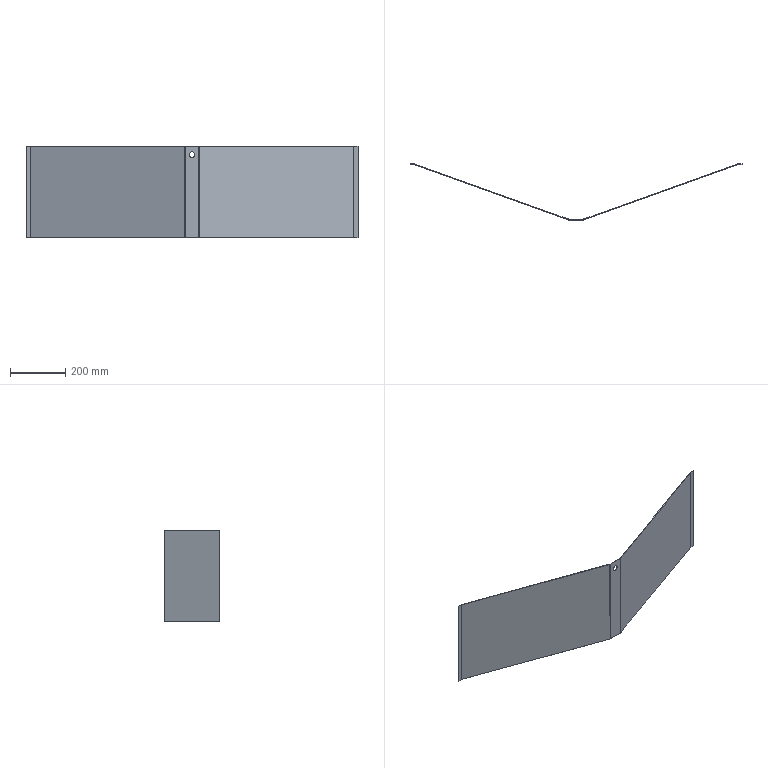Part | SolidWorks | features ICE 2, Fillet 1, FlatPattern 1, SMBaseFlange 1, SheetMetal 1 | 1 solid | 40 faces | box 1200 x 202 x 330 mm | volume 837082 mm3 | plane 30 | cylinder 10 | commonest cylinder face diameters 2 x4 6 x4 20 x2
STEP:
#1=CARTESIAN_POINT('',(600.,-200.,290.));
#2=VERTEX_POINT('',#1);
#3=CARTESIAN_POINT('',(600.,-200.,310.));
#4=VERTEX_POINT('',#3);
#5=CARTESIAN_POINT('',(600.,-200.,300.));
#6=DIRECTION('',(0.,1.,0.));
#7=DIRECTION('',(0.,0.,1.));
#8=AXIS2_PLACEMENT_3D('',#5,#6,#7);
#9=CIRCLE('',#8,10.);
#10=EDGE_CURVE('',#2,#4,#9,.T.);
#11=ORIENTED_EDGE('',*,*,#10,.T.);
#12=CARTESIAN_POINT('',(600.,-202.,310.));
#13=VERTEX_POINT('',#12);
#14=CARTESIAN_POINT('',(600.,-192.,310.));
#15=DIRECTION('',(0.,-1.,0.));
#16=VECTOR('',#15,1000.);
#17=LINE('',#14,#16);
#18=EDGE_CURVE('',#4,#13,#17,.T.);
#19=ORIENTED_EDGE('',*,*,#18,.T.);
#20=CARTESIAN_POINT('',(600.,-202.,290.));
#21=VERTEX_POINT('',#20);
#22=CARTESIAN_POINT('',(600.,-202.,300.));
#23=DIRECTION('',(0.,-1.,0.));
#24=DIRECTION('',(0.,0.,-1.));
#25=AXIS2_PLACEMENT_3D('',#22,#23,#24);
#26=CIRCLE('',#25,10.);
#27=EDGE_CURVE('',#13,#21,#26,.T.);
#28=ORIENTED_EDGE('',*,*,#27,.T.);
#29=CARTESIAN_POINT('',(600.,-192.,290.));
#30=DIRECTION('',(0.,-1.,0.));
#31=VECTOR('',#30,1000.);
#32=LINE('',#29,#31);
#33=EDGE_CURVE('',#2,#21,#32,.T.);
#34=ORIENTED_EDGE('',*,*,#33,.F.);
#35=EDGE_LOOP('',(#11,#19,#28,#34));
#36=FACE_OUTER_BOUND('',#35,.T.);
#37=CARTESIAN_POINT('',(600.,-192.,300.));
#38=DIRECTION('',(0.,-1.,0.));
#39=DIRECTION('',(0.,0.,-1.));
#40=AXIS2_PLACEMENT_3D('',#37,#38,#39);
#41=CYLINDRICAL_SURFACE('',#40,10.);
#42=ADVANCED_FACE('',(#36),#41,.F.);
#43=CARTESIAN_POINT('',(15.489,-0.1748,330.));
#44=VERTEX_POINT('',#43);
#45=CARTESIAN_POINT('',(14.817,-2.058,330.));
#46=VERTEX_POINT('',#45);
#47=CARTESIAN_POINT('',(15.489,-0.1748,330.));
#48=DIRECTION('',(-0.3363,-0.9417,0.));
#49=VECTOR('',#48,1000.);
#50=LINE('',#47,#49);
#51=EDGE_CURVE('',#44,#46,#50,.T.);
#52=ORIENTED_EDGE('',*,*,#51,.F.);
#53=CARTESIAN_POINT('',(14.48,0.,330.));
#54=VERTEX_POINT('',#53);
#55=CARTESIAN_POINT('',(14.48,-3.,330.));
#56=DIRECTION('',(0.,0.,-1.));
#57=DIRECTION('',(1.,0.,0.));
#58=AXIS2_PLACEMENT_3D('',#55,#56,#57);
#59=CIRCLE('',#58,3.);
#60=EDGE_CURVE('',#54,#44,#59,.T.);
#61=ORIENTED_EDGE('',*,*,#60,.F.);
#62=CARTESIAN_POINT('',(14.48,-2.,330.));
#63=VERTEX_POINT('',#62);
#64=CARTESIAN_POINT('',(14.48,-2.,330.));
#65=DIRECTION('',(0.,1.,0.));
#66=VECTOR('',#65,1000.);
#67=LINE('',#64,#66);
#68=EDGE_CURVE('',#63,#54,#67,.T.);
#69=ORIENTED_EDGE('',*,*,#68,.F.);
#70=CARTESIAN_POINT('',(14.48,-3.,330.));
#71=DIRECTION('',(0.,0.,-1.));
#72=DIRECTION('',(1.,0.,0.));
#73=AXIS2_PLACEMENT_3D('',#70,#71,#72);
#74=CIRCLE('',#73,1.);
#75=EDGE_CURVE('',#63,#46,#74,.T.);
#76=ORIENTED_EDGE('',*,*,#75,.T.);
#77=EDGE_LOOP('',(#52,#61,#69,#76));
#78=FACE_OUTER_BOUND('',#77,.T.);
#79=CARTESIAN_POINT('',(15.489,-0.1748,330.));
#80=DIRECTION('',(0.,0.,1.));
#81=DIRECTION('',(1.,0.,0.));
#82=AXIS2_PLACEMENT_3D('',#79,#80,#81);
#83=PLANE('',#82);
#84=ADVANCED_FACE('',(#78),#83,.T.);
#85=CARTESIAN_POINT('',(574.837,-199.942,330.));
#86=VERTEX_POINT('',#85);
#87=CARTESIAN_POINT('',(15.,0.,330.));
#88=DIRECTION('',(0.9417,-0.3363,0.));
#89=VECTOR('',#88,1000.);
#90=LINE('',#87,#89);
#91=EDGE_CURVE('',#44,#86,#90,.T.);
#92=ORIENTED_EDGE('',*,*,#91,.F.);
#93=ORIENTED_EDGE('',*,*,#51,.T.);
#94=CARTESIAN_POINT('',(574.164,-201.825,330.));
#95=VERTEX_POINT('',#94);
#96=CARTESIAN_POINT('',(14.327,-1.883,330.));
#97=DIRECTION('',(0.9417,-0.3363,0.));
#98=VECTOR('',#97,1000.);
#99=LINE('',#96,#98);
#100=EDGE_CURVE('',#46,#95,#99,.T.);
#101=ORIENTED_EDGE('',*,*,#100,.T.);
#102=CARTESIAN_POINT('',(574.164,-201.825,330.));
#103=DIRECTION('',(0.3363,0.9417,0.));
#104=VECTOR('',#103,1000.);
#105=LINE('',#102,#104);
#106=EDGE_CURVE('',#95,#86,#105,.T.);
#107=ORIENTED_EDGE('',*,*,#106,.T.);
#108=EDGE_LOOP('',(#92,#93,#101,#107));
#109=FACE_OUTER_BOUND('',#108,.T.);
#110=CARTESIAN_POINT('',(14.48,-2.,330.));
#111=DIRECTION('',(0.,0.,1.));
#112=DIRECTION('',(1.,0.,0.));
#113=AXIS2_PLACEMENT_3D('',#110,#111,#112);
#114=PLANE('',#113);
#115=ADVANCED_FACE('',(#109),#114,.T.);
#116=CARTESIAN_POINT('',(14.48,0.,0.));
#117=VERTEX_POINT('',#116);
#118=CARTESIAN_POINT('',(14.48,-2.,0.));
#119=VERTEX_POINT('',#118);
#120=CARTESIAN_POINT('',(14.48,0.,0.));
#121=DIRECTION('',(0.,-1.,0.));
#122=VECTOR('',#121,1000.);
#123=LINE('',#120,#122);
#124=EDGE_CURVE('',#117,#119,#123,.T.);
#125=ORIENTED_EDGE('',*,*,#124,.F.);
#126=CARTESIAN_POINT('',(15.489,-0.1748,0.));
#127=VERTEX_POINT('',#126);
#128=CARTESIAN_POINT('',(14.48,-3.,0.));
#129=DIRECTION('',(0.,0.,-1.));
#130=DIRECTION('',(1.,0.,0.));
#131=AXIS2_PLACEMENT_3D('',#128,#129,#130);
#132=CIRCLE('',#131,3.);
#133=EDGE_CURVE('',#117,#127,#132,.T.);
#134=ORIENTED_EDGE('',*,*,#133,.T.);
#135=CARTESIAN_POINT('',(14.817,-2.058,0.));
#136=VERTEX_POINT('',#135);
#137=CARTESIAN_POINT('',(14.817,-2.058,0.));
#138=DIRECTION('',(0.3363,0.9417,0.));
#139=VECTOR('',#138,1000.);
#140=LINE('',#137,#139);
#141=EDGE_CURVE('',#136,#127,#140,.T.);
#142=ORIENTED_EDGE('',*,*,#141,.F.);
#143=CARTESIAN_POINT('',(14.48,-3.,0.));
#144=DIRECTION('',(0.,0.,-1.));
#145=DIRECTION('',(1.,0.,0.));
#146=AXIS2_PLACEMENT_3D('',#143,#144,#145);
#147=CIRCLE('',#146,1.);
#148=EDGE_CURVE('',#119,#136,#147,.T.);
#149=ORIENTED_EDGE('',*,*,#148,.F.);
#150=EDGE_LOOP('',(#125,#134,#142,#149));
#151=FACE_OUTER_BOUND('',#150,.T.);
#152=CARTESIAN_POINT('',(14.48,0.,0.));
#153=DIRECTION('',(0.,0.,-1.));
#154=DIRECTION('',(-1.,0.,0.));
#155=AXIS2_PLACEMENT_3D('',#152,#153,#154);
#156=PLANE('',#155);
#157=ADVANCED_FACE('',(#151),#156,.T.);
#158=CARTESIAN_POINT('',(0.,0.,0.));
#159=VERTEX_POINT('',#158);
#160=CARTESIAN_POINT('',(0.,0.,0.));
#161=DIRECTION('',(1.,0.,0.));
#162=VECTOR('',#161,1000.);
#163=LINE('',#160,#162);
#164=EDGE_CURVE('',#159,#117,#163,.T.);
#165=ORIENTED_EDGE('',*,*,#164,.T.);
#166=ORIENTED_EDGE('',*,*,#124,.T.);
#167=CARTESIAN_POINT('',(0.,-2.,0.));
#168=VERTEX_POINT('',#167);
#169=CARTESIAN_POINT('',(0.,-2.,0.));
#170=DIRECTION('',(1.,0.,0.));
#171=VECTOR('',#170,1000.);
#172=LINE('',#169,#171);
#173=EDGE_CURVE('',#168,#119,#172,.T.);
#174=ORIENTED_EDGE('',*,*,#173,.F.);
#175=CARTESIAN_POINT('',(0.,-2.,0.));
#176=DIRECTION('',(0.,1.,0.));
#177=VECTOR('',#176,1000.);
#178=LINE('',#175,#177);
#179=EDGE_CURVE('',#168,#159,#178,.T.);
#180=ORIENTED_EDGE('',*,*,#179,.T.);
#181=EDGE_LOOP('',(#165,#166,#174,#180));
#182=FACE_OUTER_BOUND('',#181,.T.);
#183=CARTESIAN_POINT('',(14.817,-2.058,0.));
#184=DIRECTION('',(0.,0.,-1.));
#185=DIRECTION('',(-1.,0.,0.));
#186=AXIS2_PLACEMENT_3D('',#183,#184,#185);
#187=PLANE('',#186);
#188=ADVANCED_FACE('',(#182),#187,.T.);
#189=CARTESIAN_POINT('',(575.173,-200.,330.));
#190=VERTEX_POINT('',#189);
#191=CARTESIAN_POINT('',(575.173,-202.,330.));
#192=VERTEX_POINT('',#191);
#193=CARTESIAN_POINT('',(575.173,-200.,330.));
#194=DIRECTION('',(0.,-1.,0.));
#195=VECTOR('',#194,1000.);
#196=LINE('',#193,#195);
#197=EDGE_CURVE('',#190,#192,#196,.T.);
#198=ORIENTED_EDGE('',*,*,#197,.F.);
#199=CARTESIAN_POINT('',(575.173,-199.,330.));
#200=DIRECTION('',(0.,0.,1.));
#201=DIRECTION('',(-1.,0.,0.));
#202=AXIS2_PLACEMENT_3D('',#199,#200,#201);
#203=CIRCLE('',#202,1.);
#204=EDGE_CURVE('',#86,#190,#203,.T.);
#205=ORIENTED_EDGE('',*,*,#204,.F.);
#206=ORIENTED_EDGE('',*,*,#106,.F.);
#207=CARTESIAN_POINT('',(575.173,-199.,330.));
#208=DIRECTION('',(0.,0.,1.));
#209=DIRECTION('',(1.,0.,0.));
#210=AXIS2_PLACEMENT_3D('',#207,#208,#209);
#211=CIRCLE('',#210,3.);
#212=EDGE_CURVE('',#95,#192,#211,.T.);
#213=ORIENTED_EDGE('',*,*,#212,.T.);
#214=EDGE_LOOP('',(#198,#205,#206,#213));
#215=FACE_OUTER_BOUND('',#214,.T.);
#216=CARTESIAN_POINT('',(575.173,-200.,330.));
#217=DIRECTION('',(0.,0.,1.));
#218=DIRECTION('',(1.,0.,0.));
#219=AXIS2_PLACEMENT_3D('',#216,#217,#218);
#220=PLANE('',#219);
#221=ADVANCED_FACE('',(#215),#220,.T.);
#222=CARTESIAN_POINT('',(624.827,-200.,330.));
#223=VERTEX_POINT('',#222);
#224=CARTESIAN_POINT('',(575.,-200.,330.));
#225=DIRECTION('',(1.,0.,0.));
#226=VECTOR('',#225,1000.);
#227=LINE('',#224,#226);
#228=EDGE_CURVE('',#190,#223,#227,.T.);
#229=ORIENTED_EDGE('',*,*,#228,.F.);
#230=ORIENTED_EDGE('',*,*,#197,.T.);
#231=CARTESIAN_POINT('',(624.827,-202.,330.));
#232=VERTEX_POINT('',#231);
#233=CARTESIAN_POINT('',(575.,-202.,330.));
#234=DIRECTION('',(1.,0.,0.));
#235=VECTOR('',#234,1000.);
#236=LINE('',#233,#235);
#237=EDGE_CURVE('',#192,#232,#236,.T.);
#238=ORIENTED_EDGE('',*,*,#237,.T.);
#239=CARTESIAN_POINT('',(624.827,-202.,330.));
#240=DIRECTION('',(0.,1.,0.));
#241=VECTOR('',#240,1000.);
#242=LINE('',#239,#241);
#243=EDGE_CURVE('',#232,#223,#242,.T.);
#244=ORIENTED_EDGE('',*,*,#243,.T.);
#245=EDGE_LOOP('',(#229,#230,#238,#244));
#246=FACE_OUTER_BOUND('',#245,.T.);
#247=CARTESIAN_POINT('',(574.164,-201.825,330.));
#248=DIRECTION('',(0.,0.,1.));
#249=DIRECTION('',(1.,0.,0.));
#250=AXIS2_PLACEMENT_3D('',#247,#248,#249);
#251=PLANE('',#250);
#252=ADVANCED_FACE('',(#246),#251,.T.);
#253=CARTESIAN_POINT('',(574.837,-199.942,0.));
#254=VERTEX_POINT('',#253);
#255=CARTESIAN_POINT('',(574.164,-201.825,0.));
#256=VERTEX_POINT('',#255);
#257=CARTESIAN_POINT('',(574.837,-199.942,0.));
#258=DIRECTION('',(-0.3363,-0.9417,0.));
#259=VECTOR('',#258,1000.);
#260=LINE('',#257,#259);
#261=EDGE_CURVE('',#254,#256,#260,.T.);
#262=ORIENTED_EDGE('',*,*,#261,.F.);
#263=CARTESIAN_POINT('',(575.173,-200.,0.));
#264=VERTEX_POINT('',#263);
#265=CARTESIAN_POINT('',(575.173,-199.,0.));
#266=DIRECTION('',(0.,0.,1.));
#267=DIRECTION('',(-1.,0.,0.));
#268=AXIS2_PLACEMENT_3D('',#265,#266,#267);
#269=CIRCLE('',#268,1.);
#270=EDGE_CURVE('',#254,#264,#269,.T.);
#271=ORIENTED_EDGE('',*,*,#270,.T.);
#272=CARTESIAN_POINT('',(575.173,-202.,0.));
#273=VERTEX_POINT('',#272);
#274=CARTESIAN_POINT('',(575.173,-202.,0.));
#275=DIRECTION('',(0.,1.,0.));
#276=VECTOR('',#275,1000.);
#277=LINE('',#274,#276);
#278=EDGE_CURVE('',#273,#264,#277,.T.);
#279=ORIENTED_EDGE('',*,*,#278,.F.);
#280=CARTESIAN_POINT('',(575.173,-199.,0.));
#281=DIRECTION('',(0.,0.,1.));
#282=DIRECTION('',(1.,0.,0.));
#283=AXIS2_PLACEMENT_3D('',#280,#281,#282);
#284=CIRCLE('',#283,3.);
#285=EDGE_CURVE('',#256,#273,#284,.T.);
#286=ORIENTED_EDGE('',*,*,#285,.F.);
#287=EDGE_LOOP('',(#262,#271,#279,#286));
#288=FACE_OUTER_BOUND('',#287,.T.);
#289=CARTESIAN_POINT('',(574.837,-199.942,0.));
#290=DIRECTION('',(0.,0.,-1.));
#291=DIRECTION('',(-1.,0.,0.));
#292=AXIS2_PLACEMENT_3D('',#289,#290,#291);
#293=PLANE('',#292);
#294=ADVANCED_FACE('',(#288),#293,.T.);
#295=CARTESIAN_POINT('',(15.,0.,0.));
#296=DIRECTION('',(0.9417,-0.3363,0.));
#297=VECTOR('',#296,1000.);
#298=LINE('',#295,#297);
#299=EDGE_CURVE('',#127,#254,#298,.T.);
#300=ORIENTED_EDGE('',*,*,#299,.T.);
#301=ORIENTED_EDGE('',*,*,#261,.T.);
#302=CARTESIAN_POINT('',(14.327,-1.883,0.));
#303=DIRECTION('',(0.9417,-0.3363,0.));
#304=VECTOR('',#303,1000.);
#305=LINE('',#302,#304);
#306=EDGE_CURVE('',#136,#256,#305,.T.);
#307=ORIENTED_EDGE('',*,*,#306,.F.);
#308=ORIENTED_EDGE('',*,*,#141,.T.);
#309=EDGE_LOOP('',(#300,#301,#307,#308));
#310=FACE_OUTER_BOUND('',#309,.T.);
#311=CARTESIAN_POINT('',(575.173,-202.,0.));
#312=DIRECTION('',(0.,0.,-1.));
#313=DIRECTION('',(-1.,0.,0.));
#314=AXIS2_PLACEMENT_3D('',#311,#312,#313);
#315=PLANE('',#314);
#316=ADVANCED_FACE('',(#310),#315,.T.);
#317=CARTESIAN_POINT('',(625.163,-199.942,330.));
#318=VERTEX_POINT('',#317);
#319=CARTESIAN_POINT('',(625.836,-201.825,330.));
#320=VERTEX_POINT('',#319);
#321=CARTESIAN_POINT('',(625.163,-199.942,330.));
#322=DIRECTION('',(0.3363,-0.9417,0.));
#323=VECTOR('',#322,1000.);
#324=LINE('',#321,#323);
#325=EDGE_CURVE('',#318,#320,#324,.T.);
#326=ORIENTED_EDGE('',*,*,#325,.F.);
#327=CARTESIAN_POINT('',(624.827,-199.,330.));
#328=DIRECTION('',(0.,0.,1.));
#329=DIRECTION('',(-1.,0.,0.));
#330=AXIS2_PLACEMENT_3D('',#327,#328,#329);
#331=CIRCLE('',#330,1.);
#332=EDGE_CURVE('',#223,#318,#331,.T.);
#333=ORIENTED_EDGE('',*,*,#332,.F.);
#334=ORIENTED_EDGE('',*,*,#243,.F.);
#335=CARTESIAN_POINT('',(624.827,-199.,330.));
#336=DIRECTION('',(0.,0.,1.));
#337=DIRECTION('',(1.,0.,0.));
#338=AXIS2_PLACEMENT_3D('',#335,#336,#337);
#339=CIRCLE('',#338,3.);
#340=EDGE_CURVE('',#232,#320,#339,.T.);
#341=ORIENTED_EDGE('',*,*,#340,.T.);
#342=EDGE_LOOP('',(#326,#333,#334,#341));
#343=FACE_OUTER_BOUND('',#342,.T.);
#344=CARTESIAN_POINT('',(625.163,-199.942,330.));
#345=DIRECTION('',(0.,0.,1.));
#346=DIRECTION('',(1.,0.,0.));
#347=AXIS2_PLACEMENT_3D('',#344,#345,#346);
#348=PLANE('',#347);
#349=ADVANCED_FACE('',(#343),#348,.T.);
#350=CARTESIAN_POINT('',(1184.511,-0.1748,330.));
#351=VERTEX_POINT('',#350);
#352=CARTESIAN_POINT('',(625.,-200.,330.));
#353=DIRECTION('',(0.9417,0.3363,0.));
#354=VECTOR('',#353,1000.);
#355=LINE('',#352,#354);
#356=EDGE_CURVE('',#318,#351,#355,.T.);
#357=ORIENTED_EDGE('',*,*,#356,.F.);
#358=ORIENTED_EDGE('',*,*,#325,.T.);
#359=CARTESIAN_POINT('',(1185.183,-2.058,330.));
#360=VERTEX_POINT('',#359);
#361=CARTESIAN_POINT('',(625.673,-201.883,330.));
#362=DIRECTION('',(0.9417,0.3363,0.));
#363=VECTOR('',#362,1000.);
#364=LINE('',#361,#363);
#365=EDGE_CURVE('',#320,#360,#364,.T.);
#366=ORIENTED_EDGE('',*,*,#365,.T.);
#367=CARTESIAN_POINT('',(1185.183,-2.058,330.));
#368=DIRECTION('',(-0.3363,0.9417,0.));
#369=VECTOR('',#368,1000.);
#370=LINE('',#367,#369);
#371=EDGE_CURVE('',#360,#351,#370,.T.);
#372=ORIENTED_EDGE('',*,*,#371,.T.);
#373=EDGE_LOOP('',(#357,#358,#366,#372));
#374=FACE_OUTER_BOUND('',#373,.T.);
#375=CARTESIAN_POINT('',(624.827,-202.,330.));
#376=DIRECTION('',(0.,0.,1.));
#377=DIRECTION('',(1.,0.,0.));
#378=AXIS2_PLACEMENT_3D('',#375,#376,#377);
#379=PLANE('',#378);
#380=ADVANCED_FACE('',(#374),#379,.T.);
#381=CARTESIAN_POINT('',(624.827,-200.,0.));
#382=VERTEX_POINT('',#381);
#383=CARTESIAN_POINT('',(624.827,-202.,0.));
#384=VERTEX_POINT('',#383);
#385=CARTESIAN_POINT('',(624.827,-200.,0.));
#386=DIRECTION('',(0.,-1.,0.));
#387=VECTOR('',#386,1000.);
#388=LINE('',#385,#387);
#389=EDGE_CURVE('',#382,#384,#388,.T.);
#390=ORIENTED_EDGE('',*,*,#389,.F.);
#391=CARTESIAN_POINT('',(625.163,-199.942,0.));
#392=VERTEX_POINT('',#391);
#393=CARTESIAN_POINT('',(624.827,-199.,0.));
#394=DIRECTION('',(0.,0.,1.));
#395=DIRECTION('',(-1.,0.,0.));
#396=AXIS2_PLACEMENT_3D('',#393,#394,#395);
#397=CIRCLE('',#396,1.);
#398=EDGE_CURVE('',#382,#392,#397,.T.);
#399=ORIENTED_EDGE('',*,*,#398,.T.);
#400=CARTESIAN_POINT('',(625.836,-201.825,0.));
#401=VERTEX_POINT('',#400);
#402=CARTESIAN_POINT('',(625.836,-201.825,0.));
#403=DIRECTION('',(-0.3363,0.9417,0.));
#404=VECTOR('',#403,1000.);
#405=LINE('',#402,#404);
#406=EDGE_CURVE('',#401,#392,#405,.T.);
#407=ORIENTED_EDGE('',*,*,#406,.F.);
#408=CARTESIAN_POINT('',(624.827,-199.,0.));
#409=DIRECTION('',(0.,0.,1.));
#410=DIRECTION('',(1.,0.,0.));
#411=AXIS2_PLACEMENT_3D('',#408,#409,#410);
#412=CIRCLE('',#411,3.);
#413=EDGE_CURVE('',#384,#401,#412,.T.);
#414=ORIENTED_EDGE('',*,*,#413,.F.);
#415=EDGE_LOOP('',(#390,#399,#407,#414));
#416=FACE_OUTER_BOUND('',#415,.T.);
#417=CARTESIAN_POINT('',(624.827,-200.,0.));
#418=DIRECTION('',(0.,0.,-1.));
#419=DIRECTION('',(-1.,0.,0.));
#420=AXIS2_PLACEMENT_3D('',#417,#418,#419);
#421=PLANE('',#420);
#422=ADVANCED_FACE('',(#416),#421,.T.);
#423=CARTESIAN_POINT('',(575.,-200.,0.));
#424=DIRECTION('',(1.,0.,0.));
#425=VECTOR('',#424,1000.);
#426=LINE('',#423,#425);
#427=EDGE_CURVE('',#264,#382,#426,.T.);
#428=ORIENTED_EDGE('',*,*,#427,.T.);
#429=ORIENTED_EDGE('',*,*,#389,.T.);
#430=CARTESIAN_POINT('',(575.,-202.,0.));
#431=DIRECTION('',(1.,0.,0.));
#432=VECTOR('',#431,1000.);
#433=LINE('',#430,#432);
#434=EDGE_CURVE('',#273,#384,#433,.T.);
#435=ORIENTED_EDGE('',*,*,#434,.F.);
#436=ORIENTED_EDGE('',*,*,#278,.T.);
#437=EDGE_LOOP('',(#428,#429,#435,#436));
#438=FACE_OUTER_BOUND('',#437,.T.);
#439=CARTESIAN_POINT('',(625.836,-201.825,0.));
#440=DIRECTION('',(0.,0.,-1.));
#441=DIRECTION('',(-1.,0.,0.));
#442=AXIS2_PLACEMENT_3D('',#439,#440,#441);
#443=PLANE('',#442);
#444=ADVANCED_FACE('',(#438),#443,.T.);
#445=CARTESIAN_POINT('',(1185.52,0.,330.));
#446=VERTEX_POINT('',#445);
#447=CARTESIAN_POINT('',(1185.52,-2.,330.));
#448=VERTEX_POINT('',#447);
#449=CARTESIAN_POINT('',(1185.52,0.,330.));
#450=DIRECTION('',(0.,-1.,0.));
#451=VECTOR('',#450,1000.);
#452=LINE('',#449,#451);
#453=EDGE_CURVE('',#446,#448,#452,.T.);
#454=ORIENTED_EDGE('',*,*,#453,.F.);
#455=CARTESIAN_POINT('',(1185.52,-3.,330.));
#456=DIRECTION('',(0.,0.,-1.));
#457=DIRECTION('',(1.,0.,0.));
#458=AXIS2_PLACEMENT_3D('',#455,#456,#457);
#459=CIRCLE('',#458,3.);
#460=EDGE_CURVE('',#351,#446,#459,.T.);
#461=ORIENTED_EDGE('',*,*,#460,.F.);
#462=ORIENTED_EDGE('',*,*,#371,.F.);
#463=CARTESIAN_POINT('',(1185.52,-3.,330.));
#464=DIRECTION('',(0.,0.,-1.));
#465=DIRECTION('',(1.,0.,0.));
#466=AXIS2_PLACEMENT_3D('',#463,#464,#465);
#467=CIRCLE('',#466,1.);
#468=EDGE_CURVE('',#360,#448,#467,.T.);
#469=ORIENTED_EDGE('',*,*,#468,.T.);
#470=EDGE_LOOP('',(#454,#461,#462,#469));
#471=FACE_OUTER_BOUND('',#470,.T.);
#472=CARTESIAN_POINT('',(1185.52,0.,330.));
#473=DIRECTION('',(0.,0.,1.));
#474=DIRECTION('',(1.,0.,0.));
#475=AXIS2_PLACEMENT_3D('',#472,#473,#474);
#476=PLANE('',#475);
#477=ADVANCED_FACE('',(#471),#476,.T.);
#478=CARTESIAN_POINT('',(1200.,0.,330.));
#479=VERTEX_POINT('',#478);
#480=CARTESIAN_POINT('',(1185.,0.,330.));
#481=DIRECTION('',(1.,0.,0.));
#482=VECTOR('',#481,1000.);
#483=LINE('',#480,#482);
#484=EDGE_CURVE('',#446,#479,#483,.T.);
#485=ORIENTED_EDGE('',*,*,#484,.F.);
#486=ORIENTED_EDGE('',*,*,#453,.T.);
#487=CARTESIAN_POINT('',(1200.,-2.,330.));
#488=VERTEX_POINT('',#487);
#489=CARTESIAN_POINT('',(1185.,-2.,330.));
#490=DIRECTION('',(1.,0.,0.));
#491=VECTOR('',#490,1000.);
#492=LINE('',#489,#491);
#493=EDGE_CURVE('',#448,#488,#492,.T.);
#494=ORIENTED_EDGE('',*,*,#493,.T.);
#495=CARTESIAN_POINT('',(1200.,0.,330.));
#496=DIRECTION('',(0.,-1.,0.));
#497=VECTOR('',#496,1000.);
#498=LINE('',#495,#497);
#499=EDGE_CURVE('',#479,#488,#498,.T.);
#500=ORIENTED_EDGE('',*,*,#499,.F.);
#501=EDGE_LOOP('',(#485,#486,#494,#500));
#502=FACE_OUTER_BOUND('',#501,.T.);
#503=CARTESIAN_POINT('',(1185.183,-2.058,330.));
#504=DIRECTION('',(0.,0.,1.));
#505=DIRECTION('',(1.,0.,0.));
#506=AXIS2_PLACEMENT_3D('',#503,#504,#505);
#507=PLANE('',#506);
#508=ADVANCED_FACE('',(#502),#507,.T.);
#509=CARTESIAN_POINT('',(1184.511,-0.1748,0.));
#510=VERTEX_POINT('',#509);
#511=CARTESIAN_POINT('',(1185.183,-2.058,0.));
#512=VERTEX_POINT('',#511);
#513=CARTESIAN_POINT('',(1184.511,-0.1748,0.));
#514=DIRECTION('',(0.3363,-0.9417,0.));
#515=VECTOR('',#514,1000.);
#516=LINE('',#513,#515);
#517=EDGE_CURVE('',#510,#512,#516,.T.);
#518=ORIENTED_EDGE('',*,*,#517,.F.);
#519=CARTESIAN_POINT('',(1185.52,0.,0.));
#520=VERTEX_POINT('',#519);
#521=CARTESIAN_POINT('',(1185.52,-3.,0.));
#522=DIRECTION('',(0.,0.,-1.));
#523=DIRECTION('',(1.,0.,0.));
#524=AXIS2_PLACEMENT_3D('',#521,#522,#523);
#525=CIRCLE('',#524,3.);
#526=EDGE_CURVE('',#510,#520,#525,.T.);
#527=ORIENTED_EDGE('',*,*,#526,.T.);
#528=CARTESIAN_POINT('',(1185.52,-2.,0.));
#529=VERTEX_POINT('',#528);
#530=CARTESIAN_POINT('',(1185.52,-2.,0.));
#531=DIRECTION('',(0.,1.,0.));
#532=VECTOR('',#531,1000.);
#533=LINE('',#530,#532);
#534=EDGE_CURVE('',#529,#520,#533,.T.);
#535=ORIENTED_EDGE('',*,*,#534,.F.);
#536=CARTESIAN_POINT('',(1185.52,-3.,0.));
#537=DIRECTION('',(0.,0.,-1.));
#538=DIRECTION('',(1.,0.,0.));
#539=AXIS2_PLACEMENT_3D('',#536,#537,#538);
#540=CIRCLE('',#539,1.);
#541=EDGE_CURVE('',#512,#529,#540,.T.);
#542=ORIENTED_EDGE('',*,*,#541,.F.);
#543=EDGE_LOOP('',(#518,#527,#535,#542));
#544=FACE_OUTER_BOUND('',#543,.T.);
#545=CARTESIAN_POINT('',(1184.511,-0.1748,0.));
#546=DIRECTION('',(0.,0.,-1.));
#547=DIRECTION('',(-1.,0.,0.));
#548=AXIS2_PLACEMENT_3D('',#545,#546,#547);
#549=PLANE('',#548);
#550=ADVANCED_FACE('',(#544),#549,.T.);
#551=CARTESIAN_POINT('',(625.,-200.,0.));
#552=DIRECTION('',(0.9417,0.3363,0.));
#553=VECTOR('',#552,1000.);
#554=LINE('',#551,#553);
#555=EDGE_CURVE('',#392,#510,#554,.T.);
#556=ORIENTED_EDGE('',*,*,#555,.T.);
#557=ORIENTED_EDGE('',*,*,#517,.T.);
#558=CARTESIAN_POINT('',(625.673,-201.883,0.));
#559=DIRECTION('',(0.9417,0.3363,0.));
#560=VECTOR('',#559,1000.);
#561=LINE('',#558,#560);
#562=EDGE_CURVE('',#401,#512,#561,.T.);
#563=ORIENTED_EDGE('',*,*,#562,.F.);
#564=ORIENTED_EDGE('',*,*,#406,.T.);
#565=EDGE_LOOP('',(#556,#557,#563,#564));
#566=FACE_OUTER_BOUND('',#565,.T.);
#567=CARTESIAN_POINT('',(1185.52,-2.,0.));
#568=DIRECTION('',(0.,0.,-1.));
#569=DIRECTION('',(-1.,0.,0.));
#570=AXIS2_PLACEMENT_3D('',#567,#568,#569);
#571=PLANE('',#570);
#572=ADVANCED_FACE('',(#566),#571,.T.);
#573=CARTESIAN_POINT('',(1200.,-2.,0.));
#574=VERTEX_POINT('',#573);
#575=CARTESIAN_POINT('',(1185.,-2.,0.));
#576=DIRECTION('',(1.,0.,0.));
#577=VECTOR('',#576,1000.);
#578=LINE('',#575,#577);
#579=EDGE_CURVE('',#529,#574,#578,.T.);
#580=ORIENTED_EDGE('',*,*,#579,.T.);
#581=CARTESIAN_POINT('',(1200.,-2.,330.));
#582=DIRECTION('',(0.,0.,-1.));
#583=VECTOR('',#582,1000.);
#584=LINE('',#581,#583);
#585=EDGE_CURVE('',#488,#574,#584,.T.);
#586=ORIENTED_EDGE('',*,*,#585,.F.);
#587=ORIENTED_EDGE('',*,*,#493,.F.);
#588=CARTESIAN_POINT('',(1185.52,-2.,330.));
#589=DIRECTION('',(0.,0.,-1.));
#590=VECTOR('',#589,1000.);
#591=LINE('',#588,#590);
#592=EDGE_CURVE('',#448,#529,#591,.T.);
#593=ORIENTED_EDGE('',*,*,#592,.T.);
#594=EDGE_LOOP('',(#580,#586,#587,#593));
#595=FACE_OUTER_BOUND('',#594,.T.);
#596=CARTESIAN_POINT('',(1185.,-2.,330.));
#597=DIRECTION('',(0.,1.,0.));
#598=DIRECTION('',(0.,0.,1.));
#599=AXIS2_PLACEMENT_3D('',#596,#597,#598);
#600=PLANE('',#599);
#601=ADVANCED_FACE('',(#595),#600,.F.);
#602=CARTESIAN_POINT('',(1200.,0.,0.));
#603=VERTEX_POINT('',#602);
#604=CARTESIAN_POINT('',(1200.,0.,0.));
#605=DIRECTION('',(0.,-1.,0.));
#606=VECTOR('',#605,1000.);
#607=LINE('',#604,#606);
#608=EDGE_CURVE('',#603,#574,#607,.T.);
#609=ORIENTED_EDGE('',*,*,#608,.F.);
#610=CARTESIAN_POINT('',(1200.,0.,330.));
#611=DIRECTION('',(0.,0.,-1.));
#612=VECTOR('',#611,1000.);
#613=LINE('',#610,#612);
#614=EDGE_CURVE('',#479,#603,#613,.T.);
#615=ORIENTED_EDGE('',*,*,#614,.F.);
#616=ORIENTED_EDGE('',*,*,#499,.T.);
#617=ORIENTED_EDGE('',*,*,#585,.T.);
#618=EDGE_LOOP('',(#609,#615,#616,#617));
#619=FACE_OUTER_BOUND('',#618,.T.);
#620=CARTESIAN_POINT('',(1200.,0.,330.));
#621=DIRECTION('',(1.,0.,0.));
#622=DIRECTION('',(0.,0.,-1.));
#623=AXIS2_PLACEMENT_3D('',#620,#621,#622);
#624=PLANE('',#623);
#625=ADVANCED_FACE('',(#619),#624,.T.);
#626=CARTESIAN_POINT('',(1185.,0.,0.));
#627=DIRECTION('',(1.,0.,0.));
#628=VECTOR('',#627,1000.);
#629=LINE('',#626,#628);
#630=EDGE_CURVE('',#520,#603,#629,.T.);
#631=ORIENTED_EDGE('',*,*,#630,.F.);
#632=CARTESIAN_POINT('',(1185.52,0.,330.));
#633=DIRECTION('',(0.,0.,-1.));
#634=VECTOR('',#633,1000.);
#635=LINE('',#632,#634);
#636=EDGE_CURVE('',#446,#520,#635,.T.);
#637=ORIENTED_EDGE('',*,*,#636,.F.);
#638=ORIENTED_EDGE('',*,*,#484,.T.);
#639=ORIENTED_EDGE('',*,*,#614,.T.);
#640=EDGE_LOOP('',(#631,#637,#638,#639));
#641=FACE_OUTER_BOUND('',#640,.T.);
#642=CARTESIAN_POINT('',(1185.,0.,330.));
#643=DIRECTION('',(0.,1.,0.));
#644=DIRECTION('',(0.,0.,1.));
#645=AXIS2_PLACEMENT_3D('',#642,#643,#644);
#646=PLANE('',#645);
#647=ADVANCED_FACE('',(#641),#646,.T.);
#648=ORIENTED_EDGE('',*,*,#526,.F.);
#649=CARTESIAN_POINT('',(1184.511,-0.1748,330.));
#650=DIRECTION('',(0.,0.,-1.));
#651=VECTOR('',#650,1000.);
#652=LINE('',#649,#651);
#653=EDGE_CURVE('',#351,#510,#652,.T.);
#654=ORIENTED_EDGE('',*,*,#653,.F.);
#655=ORIENTED_EDGE('',*,*,#460,.T.);
#656=ORIENTED_EDGE('',*,*,#636,.T.);
#657=EDGE_LOOP('',(#648,#654,#655,#656));
#658=FACE_OUTER_BOUND('',#657,.T.);
#659=CARTESIAN_POINT('',(1185.52,-3.,330.));
#660=DIRECTION('',(0.,0.,-1.));
#661=DIRECTION('',(-1.,0.,0.));
#662=AXIS2_PLACEMENT_3D('',#659,#660,#661);
#663=CYLINDRICAL_SURFACE('',#662,3.);
#664=ADVANCED_FACE('',(#658),#663,.T.);
#665=ORIENTED_EDGE('',*,*,#555,.F.);
#666=CARTESIAN_POINT('',(625.163,-199.942,330.));
#667=DIRECTION('',(0.,0.,-1.));
#668=VECTOR('',#667,1000.);
#669=LINE('',#666,#668);
#670=EDGE_CURVE('',#318,#392,#669,.T.);
#671=ORIENTED_EDGE('',*,*,#670,.F.);
#672=ORIENTED_EDGE('',*,*,#356,.T.);
#673=ORIENTED_EDGE('',*,*,#653,.T.);
#674=EDGE_LOOP('',(#665,#671,#672,#673));
#675=FACE_OUTER_BOUND('',#674,.T.);
#676=CARTESIAN_POINT('',(625.,-200.,330.));
#677=DIRECTION('',(-0.3363,0.9417,0.));
#678=DIRECTION('',(-0.9417,-0.3363,0.));
#679=AXIS2_PLACEMENT_3D('',#676,#677,#678);
#680=PLANE('',#679);
#681=ADVANCED_FACE('',(#675),#680,.T.);
#682=ORIENTED_EDGE('',*,*,#398,.F.);
#683=CARTESIAN_POINT('',(624.827,-200.,330.));
#684=DIRECTION('',(0.,0.,-1.));
#685=VECTOR('',#684,1000.);
#686=LINE('',#683,#685);
#687=EDGE_CURVE('',#223,#382,#686,.T.);
#688=ORIENTED_EDGE('',*,*,#687,.F.);
#689=ORIENTED_EDGE('',*,*,#332,.T.);
#690=ORIENTED_EDGE('',*,*,#670,.T.);
#691=EDGE_LOOP('',(#682,#688,#689,#690));
#692=FACE_OUTER_BOUND('',#691,.T.);
#693=CARTESIAN_POINT('',(624.827,-199.,330.));
#694=DIRECTION('',(0.,0.,-1.));
#695=DIRECTION('',(-1.,0.,0.));
#696=AXIS2_PLACEMENT_3D('',#693,#694,#695);
#697=CYLINDRICAL_SURFACE('',#696,1.);
#698=ADVANCED_FACE('',(#692),#697,.F.);
#699=ORIENTED_EDGE('',*,*,#10,.F.);
#700=CARTESIAN_POINT('',(600.,-200.,300.));
#701=DIRECTION('',(0.,1.,0.));
#702=DIRECTION('',(0.,0.,1.));
#703=AXIS2_PLACEMENT_3D('',#700,#701,#702);
#704=CIRCLE('',#703,10.);
#705=EDGE_CURVE('',#4,#2,#704,.T.);
#706=ORIENTED_EDGE('',*,*,#705,.F.);
#707=EDGE_LOOP('',(#699,#706));
#708=FACE_BOUND('',#707,.T.);
#709=ORIENTED_EDGE('',*,*,#427,.F.);
#710=CARTESIAN_POINT('',(575.173,-200.,330.));
#711=DIRECTION('',(0.,0.,-1.));
#712=VECTOR('',#711,1000.);
#713=LINE('',#710,#712);
#714=EDGE_CURVE('',#190,#264,#713,.T.);
#715=ORIENTED_EDGE('',*,*,#714,.F.);
#716=ORIENTED_EDGE('',*,*,#228,.T.);
#717=ORIENTED_EDGE('',*,*,#687,.T.);
#718=EDGE_LOOP('',(#709,#715,#716,#717));
#719=FACE_OUTER_BOUND('',#718,.T.);
#720=CARTESIAN_POINT('',(575.,-200.,330.));
#721=DIRECTION('',(0.,1.,0.));
#722=DIRECTION('',(0.,0.,1.));
#723=AXIS2_PLACEMENT_3D('',#720,#721,#722);
#724=PLANE('',#723);
#725=ADVANCED_FACE('',(#708,#719),#724,.T.);
#726=ORIENTED_EDGE('',*,*,#270,.F.);
#727=CARTESIAN_POINT('',(574.837,-199.942,330.));
#728=DIRECTION('',(0.,0.,-1.));
#729=VECTOR('',#728,1000.);
#730=LINE('',#727,#729);
#731=EDGE_CURVE('',#86,#254,#730,.T.);
#732=ORIENTED_EDGE('',*,*,#731,.F.);
#733=ORIENTED_EDGE('',*,*,#204,.T.);
#734=ORIENTED_EDGE('',*,*,#714,.T.);
#735=EDGE_LOOP('',(#726,#732,#733,#734));
#736=FACE_OUTER_BOUND('',#735,.T.);
#737=CARTESIAN_POINT('',(575.173,-199.,330.));
#738=DIRECTION('',(0.,0.,-1.));
#739=DIRECTION('',(-1.,0.,0.));
#740=AXIS2_PLACEMENT_3D('',#737,#738,#739);
#741=CYLINDRICAL_SURFACE('',#740,1.);
#742=ADVANCED_FACE('',(#736),#741,.F.);
#743=ORIENTED_EDGE('',*,*,#299,.F.);
#744=CARTESIAN_POINT('',(15.489,-0.1748,330.));
#745=DIRECTION('',(0.,0.,-1.));
#746=VECTOR('',#745,1000.);
#747=LINE('',#744,#746);
#748=EDGE_CURVE('',#44,#127,#747,.T.);
#749=ORIENTED_EDGE('',*,*,#748,.F.);
#750=ORIENTED_EDGE('',*,*,#91,.T.);
#751=ORIENTED_EDGE('',*,*,#731,.T.);
#752=EDGE_LOOP('',(#743,#749,#750,#751));
#753=FACE_OUTER_BOUND('',#752,.T.);
#754=CARTESIAN_POINT('',(15.,0.,330.));
#755=DIRECTION('',(0.3363,0.9417,0.));
#756=DIRECTION('',(-0.9417,0.3363,0.));
#757=AXIS2_PLACEMENT_3D('',#754,#755,#756);
#758=PLANE('',#757);
#759=ADVANCED_FACE('',(#753),#758,.T.);
#760=ORIENTED_EDGE('',*,*,#133,.F.);
#761=CARTESIAN_POINT('',(14.48,0.,330.));
#762=DIRECTION('',(0.,0.,-1.));
#763=VECTOR('',#762,1000.);
#764=LINE('',#761,#763);
#765=EDGE_CURVE('',#54,#117,#764,.T.);
#766=ORIENTED_EDGE('',*,*,#765,.F.);
#767=ORIENTED_EDGE('',*,*,#60,.T.);
#768=ORIENTED_EDGE('',*,*,#748,.T.);
#769=EDGE_LOOP('',(#760,#766,#767,#768));
#770=FACE_OUTER_BOUND('',#769,.T.);
#771=CARTESIAN_POINT('',(14.48,-3.,330.));
#772=DIRECTION('',(0.,0.,-1.));
#773=DIRECTION('',(-1.,0.,0.));
#774=AXIS2_PLACEMENT_3D('',#771,#772,#773);
#775=CYLINDRICAL_SURFACE('',#774,3.);
#776=ADVANCED_FACE('',(#770),#775,.T.);
#777=ORIENTED_EDGE('',*,*,#164,.F.);
#778=CARTESIAN_POINT('',(0.,0.,330.));
#779=VERTEX_POINT('',#778);
#780=CARTESIAN_POINT('',(0.,0.,330.));
#781=DIRECTION('',(0.,0.,-1.));
#782=VECTOR('',#781,1000.);
#783=LINE('',#780,#782);
#784=EDGE_CURVE('',#779,#159,#783,.T.);
#785=ORIENTED_EDGE('',*,*,#784,.F.);
#786=CARTESIAN_POINT('',(0.,0.,330.));
#787=DIRECTION('',(1.,0.,0.));
#788=VECTOR('',#787,1000.);
#789=LINE('',#786,#788);
#790=EDGE_CURVE('',#779,#54,#789,.T.);
#791=ORIENTED_EDGE('',*,*,#790,.T.);
#792=ORIENTED_EDGE('',*,*,#765,.T.);
#793=EDGE_LOOP('',(#777,#785,#791,#792));
#794=FACE_OUTER_BOUND('',#793,.T.);
#795=CARTESIAN_POINT('',(0.,0.,330.));
#796=DIRECTION('',(0.,1.,0.));
#797=DIRECTION('',(0.,0.,1.));
#798=AXIS2_PLACEMENT_3D('',#795,#796,#797);
#799=PLANE('',#798);
#800=ADVANCED_FACE('',(#794),#799,.T.);
#801=ORIENTED_EDGE('',*,*,#179,.F.);
#802=CARTESIAN_POINT('',(0.,-2.,330.));
#803=VERTEX_POINT('',#802);
#804=CARTESIAN_POINT('',(0.,-2.,330.));
#805=DIRECTION('',(0.,0.,-1.));
#806=VECTOR('',#805,1000.);
#807=LINE('',#804,#806);
#808=EDGE_CURVE('',#803,#168,#807,.T.);
#809=ORIENTED_EDGE('',*,*,#808,.F.);
#810=CARTESIAN_POINT('',(0.,-2.,330.));
#811=DIRECTION('',(0.,1.,0.));
#812=VECTOR('',#811,1000.);
#813=LINE('',#810,#812);
#814=EDGE_CURVE('',#803,#779,#813,.T.);
#815=ORIENTED_EDGE('',*,*,#814,.T.);
#816=ORIENTED_EDGE('',*,*,#784,.T.);
#817=EDGE_LOOP('',(#801,#809,#815,#816));
#818=FACE_OUTER_BOUND('',#817,.T.);
#819=CARTESIAN_POINT('',(0.,-2.,330.));
#820=DIRECTION('',(-1.,0.,0.));
#821=DIRECTION('',(0.,0.,1.));
#822=AXIS2_PLACEMENT_3D('',#819,#820,#821);
#823=PLANE('',#822);
#824=ADVANCED_FACE('',(#818),#823,.T.);
#825=ORIENTED_EDGE('',*,*,#173,.T.);
#826=CARTESIAN_POINT('',(14.48,-2.,330.));
#827=DIRECTION('',(0.,0.,-1.));
#828=VECTOR('',#827,1000.);
#829=LINE('',#826,#828);
#830=EDGE_CURVE('',#63,#119,#829,.T.);
#831=ORIENTED_EDGE('',*,*,#830,.F.);
#832=CARTESIAN_POINT('',(0.,-2.,330.));
#833=DIRECTION('',(1.,0.,0.));
#834=VECTOR('',#833,1000.);
#835=LINE('',#832,#834);
#836=EDGE_CURVE('',#803,#63,#835,.T.);
#837=ORIENTED_EDGE('',*,*,#836,.F.);
#838=ORIENTED_EDGE('',*,*,#808,.T.);
#839=EDGE_LOOP('',(#825,#831,#837,#838));
#840=FACE_OUTER_BOUND('',#839,.T.);
#841=CARTESIAN_POINT('',(0.,-2.,330.));
#842=DIRECTION('',(0.,1.,0.));
#843=DIRECTION('',(0.,0.,1.));
#844=AXIS2_PLACEMENT_3D('',#841,#842,#843);
#845=PLANE('',#844);
#846=ADVANCED_FACE('',(#840),#845,.F.);
#847=ORIENTED_EDGE('',*,*,#148,.T.);
#848=CARTESIAN_POINT('',(14.817,-2.058,330.));
#849=DIRECTION('',(0.,0.,-1.));
#850=VECTOR('',#849,1000.);
#851=LINE('',#848,#850);
#852=EDGE_CURVE('',#46,#136,#851,.T.);
#853=ORIENTED_EDGE('',*,*,#852,.F.);
#854=ORIENTED_EDGE('',*,*,#75,.F.);
#855=ORIENTED_EDGE('',*,*,#830,.T.);
#856=EDGE_LOOP('',(#847,#853,#854,#855));
#857=FACE_OUTER_BOUND('',#856,.T.);
#858=CARTESIAN_POINT('',(14.48,-3.,330.));
#859=DIRECTION('',(0.,0.,-1.));
#860=DIRECTION('',(-1.,0.,0.));
#861=AXIS2_PLACEMENT_3D('',#858,#859,#860);
#862=CYLINDRICAL_SURFACE('',#861,1.);
#863=ADVANCED_FACE('',(#857),#862,.F.);
#864=ORIENTED_EDGE('',*,*,#306,.T.);
#865=CARTESIAN_POINT('',(574.164,-201.825,330.));
#866=DIRECTION('',(0.,0.,-1.));
#867=VECTOR('',#866,1000.);
#868=LINE('',#865,#867);
#869=EDGE_CURVE('',#95,#256,#868,.T.);
#870=ORIENTED_EDGE('',*,*,#869,.F.);
#871=ORIENTED_EDGE('',*,*,#100,.F.);
#872=ORIENTED_EDGE('',*,*,#852,.T.);
#873=EDGE_LOOP('',(#864,#870,#871,#872));
#874=FACE_OUTER_BOUND('',#873,.T.);
#875=CARTESIAN_POINT('',(14.327,-1.883,330.));
#876=DIRECTION('',(0.3363,0.9417,0.));
#877=DIRECTION('',(-0.9417,0.3363,0.));
#878=AXIS2_PLACEMENT_3D('',#875,#876,#877);
#879=PLANE('',#878);
#880=ADVANCED_FACE('',(#874),#879,.F.);
#881=ORIENTED_EDGE('',*,*,#285,.T.);
#882=CARTESIAN_POINT('',(575.173,-202.,330.));
#883=DIRECTION('',(0.,0.,-1.));
#884=VECTOR('',#883,1000.);
#885=LINE('',#882,#884);
#886=EDGE_CURVE('',#192,#273,#885,.T.);
#887=ORIENTED_EDGE('',*,*,#886,.F.);
#888=ORIENTED_EDGE('',*,*,#212,.F.);
#889=ORIENTED_EDGE('',*,*,#869,.T.);
#890=EDGE_LOOP('',(#881,#887,#888,#889));
#891=FACE_OUTER_BOUND('',#890,.T.);
#892=CARTESIAN_POINT('',(575.173,-199.,330.));
#893=DIRECTION('',(0.,0.,-1.));
#894=DIRECTION('',(-1.,0.,0.));
#895=AXIS2_PLACEMENT_3D('',#892,#893,#894);
#896=CYLINDRICAL_SURFACE('',#895,3.);
#897=ADVANCED_FACE('',(#891),#896,.T.);
#898=CARTESIAN_POINT('',(600.,-202.,300.));
#899=DIRECTION('',(0.,-1.,0.));
#900=DIRECTION('',(0.,0.,-1.));
#901=AXIS2_PLACEMENT_3D('',#898,#899,#900);
#902=CIRCLE('',#901,10.);
#903=EDGE_CURVE('',#21,#13,#902,.T.);
#904=ORIENTED_EDGE('',*,*,#903,.F.);
#905=ORIENTED_EDGE('',*,*,#27,.F.);
#906=EDGE_LOOP('',(#904,#905));
#907=FACE_BOUND('',#906,.T.);
#908=ORIENTED_EDGE('',*,*,#434,.T.);
#909=CARTESIAN_POINT('',(624.827,-202.,330.));
#910=DIRECTION('',(0.,0.,-1.));
#911=VECTOR('',#910,1000.);
#912=LINE('',#909,#911);
#913=EDGE_CURVE('',#232,#384,#912,.T.);
#914=ORIENTED_EDGE('',*,*,#913,.F.);
#915=ORIENTED_EDGE('',*,*,#237,.F.);
#916=ORIENTED_EDGE('',*,*,#886,.T.);
#917=EDGE_LOOP('',(#908,#914,#915,#916));
#918=FACE_OUTER_BOUND('',#917,.T.);
#919=CARTESIAN_POINT('',(575.,-202.,330.));
#920=DIRECTION('',(0.,1.,0.));
#921=DIRECTION('',(0.,0.,1.));
#922=AXIS2_PLACEMENT_3D('',#919,#920,#921);
#923=PLANE('',#922);
#924=ADVANCED_FACE('',(#907,#918),#923,.F.);
#925=ORIENTED_EDGE('',*,*,#413,.T.);
#926=CARTESIAN_POINT('',(625.836,-201.825,330.));
#927=DIRECTION('',(0.,0.,-1.));
#928=VECTOR('',#927,1000.);
#929=LINE('',#926,#928);
#930=EDGE_CURVE('',#320,#401,#929,.T.);
#931=ORIENTED_EDGE('',*,*,#930,.F.);
#932=ORIENTED_EDGE('',*,*,#340,.F.);
#933=ORIENTED_EDGE('',*,*,#913,.T.);
#934=EDGE_LOOP('',(#925,#931,#932,#933));
#935=FACE_OUTER_BOUND('',#934,.T.);
#936=CARTESIAN_POINT('',(624.827,-199.,330.));
#937=DIRECTION('',(0.,0.,-1.));
#938=DIRECTION('',(-1.,0.,0.));
#939=AXIS2_PLACEMENT_3D('',#936,#937,#938);
#940=CYLINDRICAL_SURFACE('',#939,3.);
#941=ADVANCED_FACE('',(#935),#940,.T.);
#942=ORIENTED_EDGE('',*,*,#562,.T.);
#943=CARTESIAN_POINT('',(1185.183,-2.058,330.));
#944=DIRECTION('',(0.,0.,-1.));
#945=VECTOR('',#944,1000.);
#946=LINE('',#943,#945);
#947=EDGE_CURVE('',#360,#512,#946,.T.);
#948=ORIENTED_EDGE('',*,*,#947,.F.);
#949=ORIENTED_EDGE('',*,*,#365,.F.);
#950=ORIENTED_EDGE('',*,*,#930,.T.);
#951=EDGE_LOOP('',(#942,#948,#949,#950));
#952=FACE_OUTER_BOUND('',#951,.T.);
#953=CARTESIAN_POINT('',(625.673,-201.883,330.));
#954=DIRECTION('',(-0.3363,0.9417,0.));
#955=DIRECTION('',(-0.9417,-0.3363,0.));
#956=AXIS2_PLACEMENT_3D('',#953,#954,#955);
#957=PLANE('',#956);
#958=ADVANCED_FACE('',(#952),#957,.F.);
#959=ORIENTED_EDGE('',*,*,#541,.T.);
#960=ORIENTED_EDGE('',*,*,#592,.F.);
#961=ORIENTED_EDGE('',*,*,#468,.F.);
#962=ORIENTED_EDGE('',*,*,#947,.T.);
#963=EDGE_LOOP('',(#959,#960,#961,#962));
#964=FACE_OUTER_BOUND('',#963,.T.);
#965=CARTESIAN_POINT('',(1185.52,-3.,330.));
#966=DIRECTION('',(0.,0.,-1.));
#967=DIRECTION('',(-1.,0.,0.));
#968=AXIS2_PLACEMENT_3D('',#965,#966,#967);
#969=CYLINDRICAL_SURFACE('',#968,1.);
#970=ADVANCED_FACE('',(#964),#969,.F.);
#971=ORIENTED_EDGE('',*,*,#836,.T.);
#972=ORIENTED_EDGE('',*,*,#68,.T.);
#973=ORIENTED_EDGE('',*,*,#790,.F.);
#974=ORIENTED_EDGE('',*,*,#814,.F.);
#975=EDGE_LOOP('',(#971,#972,#973,#974));
#976=FACE_OUTER_BOUND('',#975,.T.);
#977=CARTESIAN_POINT('',(1185.52,-3.,330.));
#978=DIRECTION('',(0.,0.,1.));
#979=DIRECTION('',(1.,0.,0.));
#980=AXIS2_PLACEMENT_3D('',#977,#978,#979);
#981=PLANE('',#980);
#982=ADVANCED_FACE('',(#976),#981,.T.);
#983=ORIENTED_EDGE('',*,*,#579,.F.);
#984=ORIENTED_EDGE('',*,*,#534,.T.);
#985=ORIENTED_EDGE('',*,*,#630,.T.);
#986=ORIENTED_EDGE('',*,*,#608,.T.);
#987=EDGE_LOOP('',(#983,#984,#985,#986));
#988=FACE_OUTER_BOUND('',#987,.T.);
#989=CARTESIAN_POINT('',(1185.52,-3.,0.));
#990=DIRECTION('',(0.,0.,1.));
#991=DIRECTION('',(1.,0.,0.));
#992=AXIS2_PLACEMENT_3D('',#989,#990,#991);
#993=PLANE('',#992);
#994=ADVANCED_FACE('',(#988),#993,.F.);
#995=ORIENTED_EDGE('',*,*,#18,.F.);
#996=ORIENTED_EDGE('',*,*,#705,.T.);
#997=ORIENTED_EDGE('',*,*,#33,.T.);
#998=ORIENTED_EDGE('',*,*,#903,.T.);
#999=EDGE_LOOP('',(#995,#996,#997,#998));
#1000=FACE_OUTER_BOUND('',#999,.T.);
#1001=CARTESIAN_POINT('',(600.,-192.,300.));
#1002=DIRECTION('',(0.,-1.,0.));
#1003=DIRECTION('',(0.,0.,-1.));
#1004=AXIS2_PLACEMENT_3D('',#1001,#1002,#1003);
#1005=CYLINDRICAL_SURFACE('',#1004,10.);
#1006=ADVANCED_FACE('',(#1000),#1005,.F.);
#1007=CLOSED_SHELL('',(#42,#84,#115,#157,#188,#221,#252,#294,#316,#349,#380,#422,#444,#477,#508,#550,#572,#601,#625,#647,#664,#681,#698,#725,#742,#759,#776,#800,#824,#846,#863,#880,#897,#924,#941,#958,#970,#982,#994,#1006));
#1008=MANIFOLD_SOLID_BREP('',#1007);
#1009=CARTESIAN_POINT('',(0.,0.,0.));
#1010=DIRECTION('',(0.,0.,1.));
#1011=DIRECTION('',(1.,0.,0.));
#1012=AXIS2_PLACEMENT_3D('',#1009,#1010,#1011);
#1013=(LENGTH_UNIT()NAMED_UNIT(*)SI_UNIT(.MILLI.,.METRE.));
#1014=UNCERTAINTY_MEASURE_WITH_UNIT(LENGTH_MEASURE(0.00001),#1013,'','');
#1015=(NAMED_UNIT(*)PLANE_ANGLE_UNIT()SI_UNIT($,.RADIAN.));
#1016=(NAMED_UNIT(*)SI_UNIT($,.STERADIAN.)SOLID_ANGLE_UNIT());
#1017=(GEOMETRIC_REPRESENTATION_CONTEXT(3)GLOBAL_UNCERTAINTY_ASSIGNED_CONTEXT((#1014))GLOBAL_UNIT_ASSIGNED_CONTEXT((#1013,#1015,#1016))REPRESENTATION_CONTEXT('',''));
#1018=ADVANCED_BREP_SHAPE_REPRESENTATION('',(#1008,#1012),#1017);